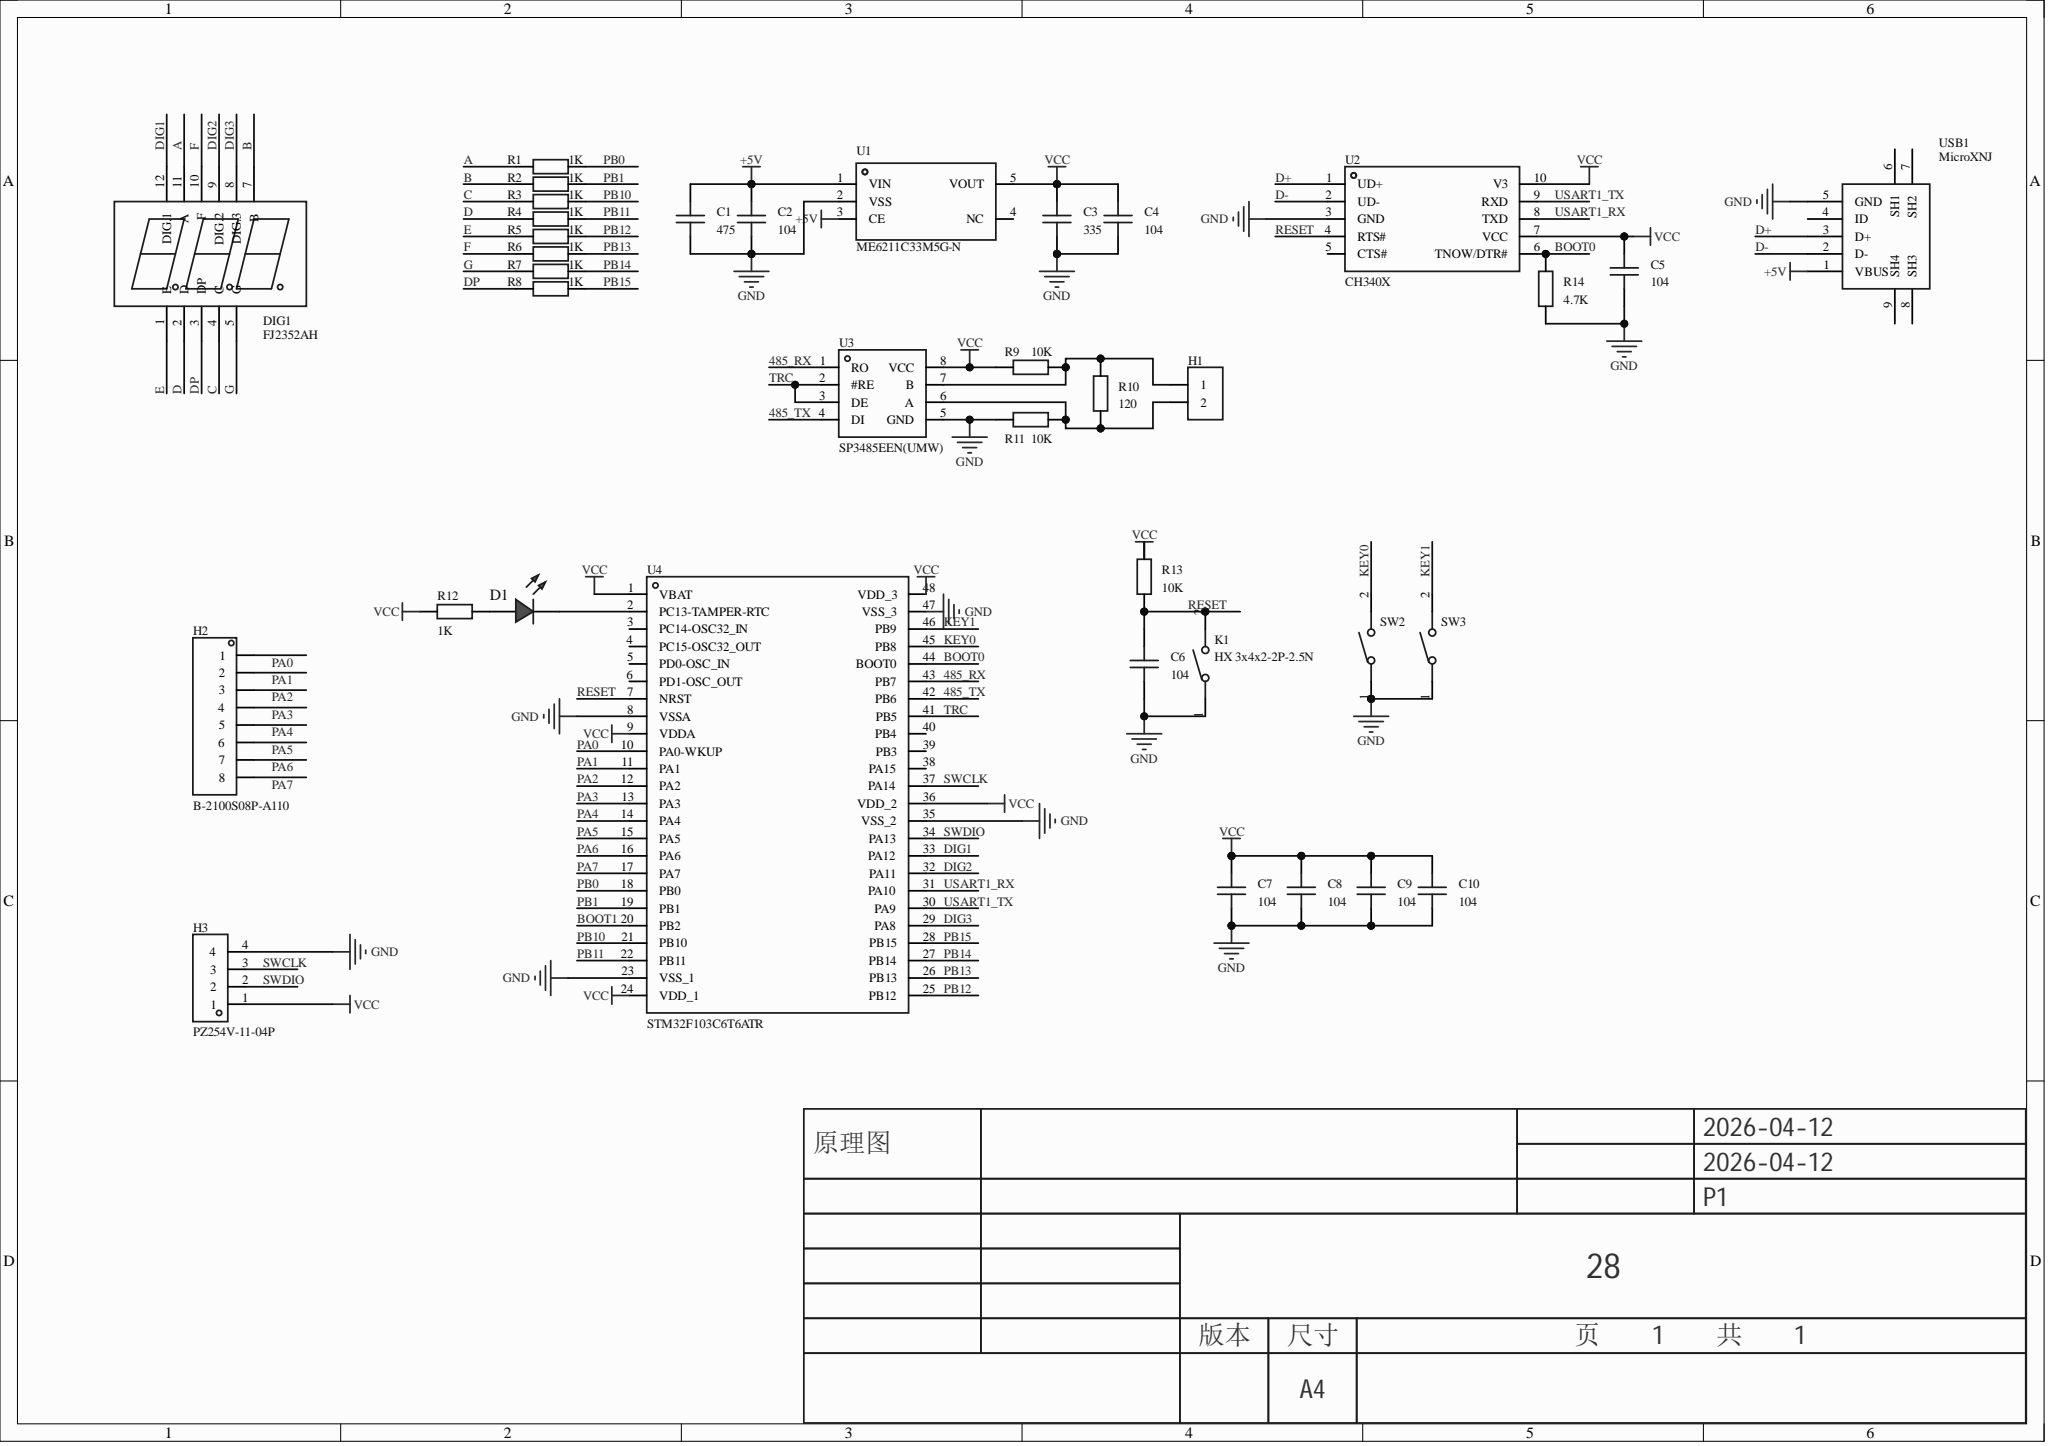Circuit board | Altium Designer | 37 parts | 47 nets
Bill of materials:
Comment,Description,Designator,Footprint,LibRef,Quantity
"475","","C1","C0805","CAP_0805","1"
"104","","C2, C4, C5, C6, C7, C8, C9, C10","C0603","CAP_0603","8"
"335","","C3","C0805","CAP_0805","1"
"","","D1","LED_0603","LED_0603-R","1"
"FJ2352AH","数码管位数:3位;字符尺寸(英寸):0.25;发光颜色:红色;LED极性:共阴极;","DIG1","LED-SEG-TH_FJ2352AH","FJ2352AH","1"
"","","H1","HDR-TH_2P-P2.54-V-F","HDR-F_2.54_1x2P","1"
"B-2100S08P-A110","插针结构:1x8P;间距:2.54mm;行距:-;圆针/方针:方针;安装方式:直插;排数:单排;总PIN位数:8P;额定电流:3A;额定电压:-;配合针长度:6mm;塑高:2.54mm;端接针长度:3mm;触头材质:黄铜;触头镀层:-;工作温度:-40℃~+105℃;颜色:黑色;","H2","HDR-TH_8P-P2.54-V-M","B-2100S08P-A110","1"
"PZ254V-11-04P","插针结构:1x4P;间距:2.54mm;行距:-;圆针/方针:方针;安装方式:直插;排数:单排;总PIN位数:4P;额定电流:3A;额定电压:250V;配合针长度:6mm;塑高:2.5mm;端接针长度:3mm;触头材质:黄铜;触头镀层:-;工作温度:-40℃~+105℃;颜色:黑色;","H3","HDR-TH_4P-P2.54-V-M","PZ254V-11-04P_C492403","1"
"HX 3x4x2-2P-2.5N","电路结构:单刀单掷;按钮形状:圆形按钮;作用力:2.5N;安装方式:立贴;开关长度:4mm;开关宽度:3mm;开关高度:2mm;带支架:不带支架;触点电流:50mA;额定电压:12V;带灯:无;工作寿命:10万次;","K1, SW2, SW3","SW-SMD_L4.0-W2.9-LS5.0","HX 3x4x2-2P-2.5N","3"
"1K","","R1, R2, R3, R4, R5, R6, R7, R8, R12","R0603","Res_0603","9"
"10K","","R9, R11, R13","R0603","Res_0603","3"
"120","","R10","R0603","Res_0603","1"
"4.7K","","R14","R0603","Res_0603","1"
"ME6211C33M5G-N","输出类型:固定;工作电压:6V;输出电压:3.3V;输出电流:500mA;电源纹波抑制比(PSRR):70dB@(1kHz);输出极性:正极;","U1","SOT-23-5_L3.0-W1.7-P0.95-LS2.8-BL","ME6211C33M5G-N","1"
"CH340X","应用功能:USB转串口；USB转并口;USB协议版本:USB 2.0;通道数:-;数据速率:2Mbps;","U2","MSOP-10_L3.0-W3.0-P0.50-LS5.0-BL","CH340X","1"
"SP3485EEN(UMW)","类型:收发器;数据速率:12Mbps;","U3","SOP-8_L5.0-W4.0-P1.27-LS6.0-BL","SP3485EEN(UMW)","1"
"STM32F103C6T6ATR","CPU内核:ARM-M3;CPU最大主频:72MHz;应用领域:-;","U4","LQFP-48_L7.0-W7.0-P0.50-LS9.0-BL","STM32F103C6T6ATR","1"
"MicroXNJ","连接器类型:Micro-B;协议标准:USB 2.0;公母:母;安装方式:卧贴;触点数量:5P;端口数量:1;额定电流 - 电源:1.8A;工作温度:-20℃~+85℃;","USB1","MICRO-USB-SMD_MICROXNJ_1","MicroXNJ","1"
Netlist (Protel format):
[
C1
C0805
475



]
[
C2
C0603
104



]
[
C3
C0805
335



]
[
C4
C0603
104



]
[
C5
C0603
104



]
[
C6
C0603
104



]
[
C7
C0603
104



]
[
C8
C0603
104



]
[
C9
C0603
104



]
[
C10
C0603
104



]
[
D1
LED_0603




]
[
DIG1
LED-SEG-TH_FJ2352AH
FJ2352AH



]
[
H1
HDR-TH_2P-P2.54-V-F




]
[
H2
HDR-TH_8P-P2.54-V-M
B-2100S08P-A110



]
[
H3
HDR-TH_4P-P2.54-V-M
PZ254V-11-04P



]
[
K1
SW-SMD_L4.0-W2.9-LS5.0
HX 3x4x2-2P-2.5N



]
[
R1
R0603
1K



]
[
R2
R0603
1K



]
[
R3
R0603
1K



]
[
R4
R0603
1K



]
[
R5
R0603
1K



]
[
R6
R0603
1K



]
[
R7
R0603
1K



]
[
R8
R0603
1K



]
[
R9
R0603
10K



]
[
R10
R0603
120



]
[
R11
R0603
10K



]
[
R12
R0603
1K



]
[
R13
R0603
10K



]
[
R14
R0603
4.7K



]
[
SW2
SW-SMD_L4.0-W2.9-LS5.0
HX 3x4x2-2P-2.5N



]
[
SW3
SW-SMD_L4.0-W2.9-LS5.0
HX 3x4x2-2P-2.5N



]
[
U1
SOT-23-5_L3.0-W1.7-P0.95-LS2.8-BL
ME6211C33M5G-N



]
[
U2
MSOP-10_L3.0-W3.0-P0.50-LS5.0-BL
CH340X



]
[
U3
SOP-8_L5.0-W4.0-P1.27-LS6.0-BL
SP3485EEN(UMW)



]
[
U4
LQFP-48_L7.0-W7.0-P0.50-LS9.0-BL
STM32F103C6T6ATR



]
[
USB1
MICRO-USB-SMD_MICROXNJ_1
MicroXNJ



]
(
VCC
C3-2
C4-2
C5-2
C7-2
C8-2
C9-2
C10-2
H3-1
R9-1
R12-1
R13-2
U1-5
U2-7
U2-10
U3-8
U4-1
U4-9
U4-24
U4-36
U4-48
)
(
USART1_TX
U2-9
U4-30
)
(
USART1_RX
U2-8
U4-31
)
(
TRC
U3-2
U3-3
U4-41
)
(
SWDIO
H3-2
U4-34
)
(
SWCLK
H3-3
U4-37
)
(
RESET
C6-2
K1-2
R13-1
U2-4
U4-7
)
(
PB15
R8-2
U4-28
)
(
PB14
R7-2
U4-27
)
(
PB13
R6-2
U4-26
)
(
PB12
R5-2
U4-25
)
(
PB11
R4-2
U4-22
)
(
PB10
R3-2
U4-21
)
(
PB1
R2-2
U4-19
)
(
PB0
R1-2
U4-18
)
(
PA7
H2-8
U4-17
)
(
PA6
H2-7
U4-16
)
(
PA5
H2-6
U4-15
)
(
PA4
H2-5
U4-14
)
(
PA3
H2-4
U4-13
)
(
PA2
H2-3
U4-12
)
(
PA1
H2-2
U4-11
)
(
PA0
H2-1
U4-10
)
(
NetH1_2
H1-2
R10-1
R11-2
U3-6
)
(
NetH1_1
H1-1
R9-2
R10-2
U3-7
)
(
NetD1_2
D1-2
R12-2
)
(
NetD1_1
D1-1
U4-2
)
(
KEY1
SW3-2
U4-46
)
(
KEY0
SW2-2
U4-45
)
(
GND
C1-1
C2-1
C3-1
C4-1
C5-1
C6-1
C7-1
C8-1
C9-1
C10-1
H3-4
K1-1
R11-1
R14-1
SW2-1
SW3-1
U1-2
U2-3
U3-5
U4-8
U4-23
U4-35
U4-47
USB1-5
)
(
G
DIG1-5
R7-1
)
(
F
DIG1-10
R6-1
)
(
E
DIG1-1
R5-1
)
(
DP
DIG1-3
R8-1
)
(
DIG3
DIG1-8
U4-29
)
(
DIG2
DIG1-9
U4-32
)
(
DIG1
DIG1-12
U4-33
)
(
D-
U2-2
USB1-2
)
(
D+
U2-1
USB1-3
)
(
D
DIG1-2
R4-1
)
(
C
DIG1-4
R3-1
)
(
BOOT0
R14-2
U2-6
U4-44
)
(
B
DIG1-7
R2-1
)
(
A
DIG1-11
R1-1
)
(
+5V
C1-2
C2-2
U1-1
U1-3
USB1-1
)
(
485_TX
U3-4
U4-42
)
(
485_RX
U3-1
U4-43
)